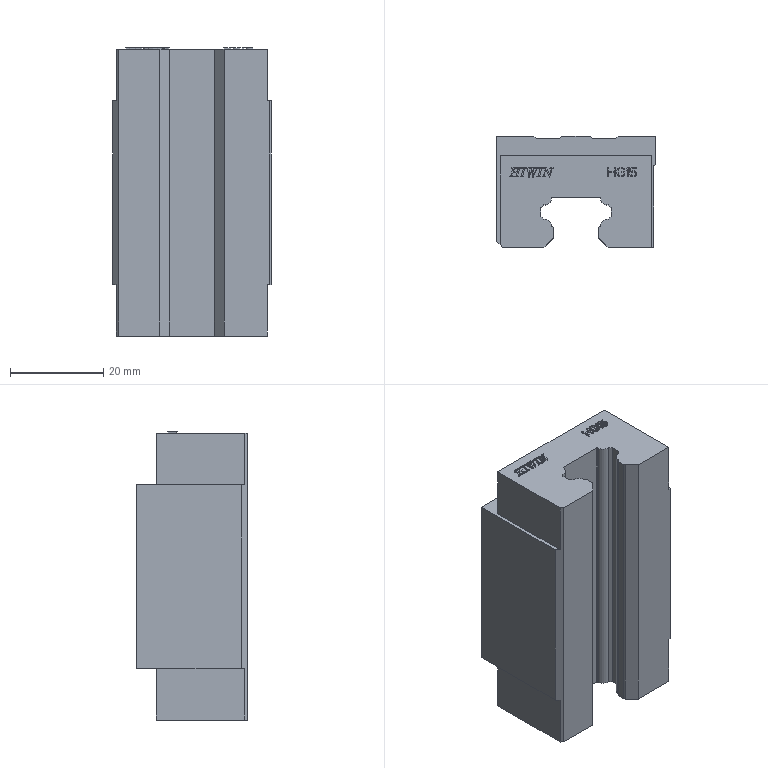Part | SolidWorks | features Chamfer 35, ICE 15, Draft 12, Fillet 3, Extrusion 1, HoleWzd 1 | 1 solid | 402 faces | box 34 x 23.7 x 61.7 mm | volume 37116 mm3 | plane 279 | spline 78 | cylinder 45 | commonest cylinder face diameters 0.072 x12 0.8 x8 4 x8 3.24 x4 1.047 x2 7.285 x2